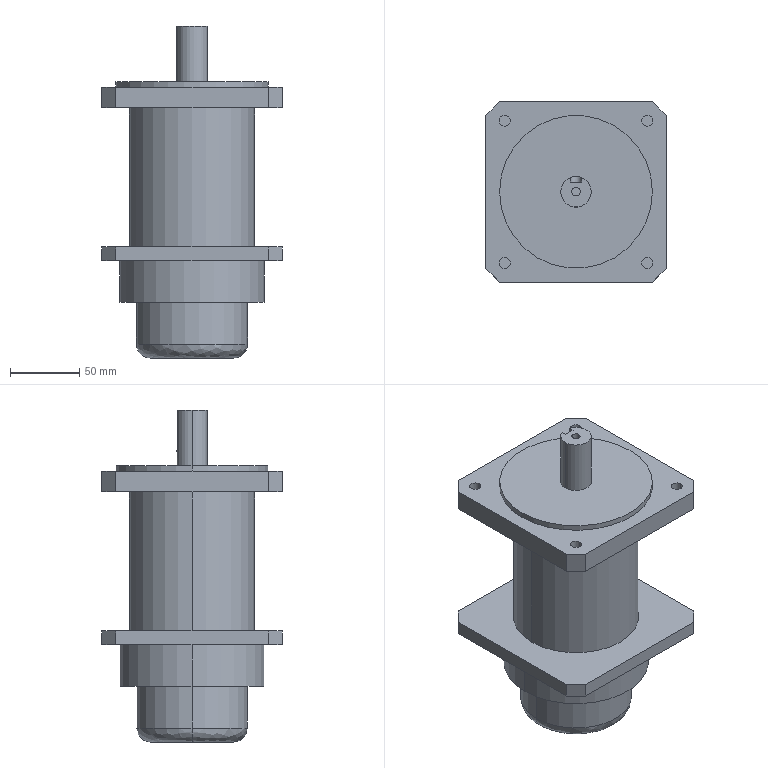Part | STEP file | Synchronous motor | 1 solid | 51 faces | box 130 x 130 x 239 mm | volume 1553555 mm3 | plane 28 | cylinder 21 | spline 2 | commonest cylinder face diameters 8 x9 6 x2 22 x2 80 x2 90 x2 104 x2